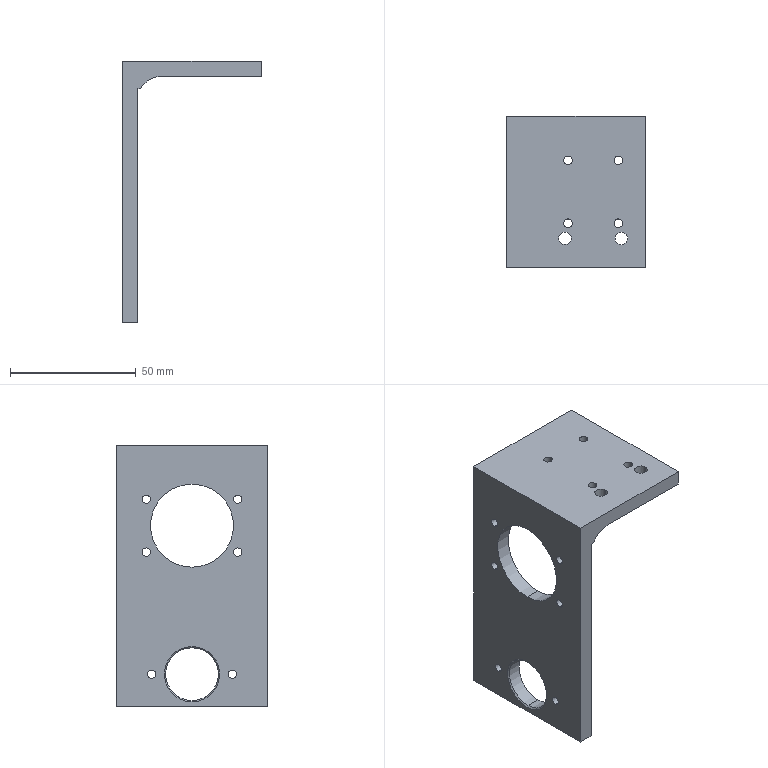Part | SolidWorks | features ICE 3, HoleWzd 2, Chamfer 1, Extrusion 1, Fillet 1 | 1 solid | 40 faces | box 55 x 60 x 104 mm | volume 48156 mm3 | cylinder 29 | plane 9 | cone 2 | commonest cylinder face diameters 3.3 x12 3.4 x8 5 x4 21 x2 33 x2 20 x1
STEP:
#1=CARTESIAN_POINT('',(0.5,30.,-101.5));
#2=VERTEX_POINT('',#1);
#3=CARTESIAN_POINT('',(0.5,30.,-80.5));
#4=VERTEX_POINT('',#3);
#5=CARTESIAN_POINT('',(0.5,30.,-91.));
#6=DIRECTION('',(-1.,0.,0.));
#7=DIRECTION('',(0.,0.,-1.));
#8=AXIS2_PLACEMENT_3D('',#5,#6,#7);
#9=CIRCLE('',#8,10.5);
#10=EDGE_CURVE('',#2,#4,#9,.T.);
#11=ORIENTED_EDGE('',*,*,#10,.F.);
#12=CARTESIAN_POINT('',(0.,30.,-102.));
#13=VERTEX_POINT('',#12);
#14=CARTESIAN_POINT('',(0.5,30.,-101.5));
#15=DIRECTION('',(-0.7071,0.,-0.7071));
#16=VECTOR('',#15,1000.);
#17=LINE('',#14,#16);
#18=EDGE_CURVE('',#2,#13,#17,.T.);
#19=ORIENTED_EDGE('',*,*,#18,.T.);
#20=CARTESIAN_POINT('',(0.,30.,-80.));
#21=VERTEX_POINT('',#20);
#22=CARTESIAN_POINT('',(0.,30.,-91.));
#23=DIRECTION('',(1.,0.,0.));
#24=DIRECTION('',(0.,0.,-1.));
#25=AXIS2_PLACEMENT_3D('',#22,#23,#24);
#26=CIRCLE('',#25,11.);
#27=EDGE_CURVE('',#21,#13,#26,.T.);
#28=ORIENTED_EDGE('',*,*,#27,.F.);
#29=CARTESIAN_POINT('',(0.5,30.,-80.5));
#30=DIRECTION('',(-0.7071,0.,0.7071));
#31=VECTOR('',#30,1000.);
#32=LINE('',#29,#31);
#33=EDGE_CURVE('',#4,#21,#32,.T.);
#34=ORIENTED_EDGE('',*,*,#33,.F.);
#35=EDGE_LOOP('',(#11,#19,#28,#34));
#36=FACE_OUTER_BOUND('',#35,.T.);
#37=CARTESIAN_POINT('',(0.5,30.,-91.));
#38=DIRECTION('',(-1.,0.,0.));
#39=DIRECTION('',(0.,0.,1.));
#40=AXIS2_PLACEMENT_3D('',#37,#38,#39);
#41=CONICAL_SURFACE('',#40,10.5,0.7854);
#42=ADVANCED_FACE('',(#36),#41,.F.);
#43=CARTESIAN_POINT('',(6.,11.813,-19.85));
#44=VERTEX_POINT('',#43);
#45=CARTESIAN_POINT('',(6.,11.813,-23.15));
#46=VERTEX_POINT('',#45);
#47=CARTESIAN_POINT('',(6.,11.813,-21.5));
#48=DIRECTION('',(1.,0.,0.));
#49=DIRECTION('',(0.,0.,-1.));
#50=AXIS2_PLACEMENT_3D('',#47,#48,#49);
#51=CIRCLE('',#50,1.65);
#52=EDGE_CURVE('',#44,#46,#51,.T.);
#53=ORIENTED_EDGE('',*,*,#52,.T.);
#54=CARTESIAN_POINT('',(0.,11.813,-23.15));
#55=VERTEX_POINT('',#54);
#56=CARTESIAN_POINT('',(0.,11.813,-23.15));
#57=DIRECTION('',(-1.,0.,0.));
#58=VECTOR('',#57,1000.);
#59=LINE('',#56,#58);
#60=EDGE_CURVE('',#46,#55,#59,.T.);
#61=ORIENTED_EDGE('',*,*,#60,.T.);
#62=CARTESIAN_POINT('',(0.,11.813,-19.85));
#63=VERTEX_POINT('',#62);
#64=CARTESIAN_POINT('',(0.,11.813,-21.5));
#65=DIRECTION('',(-1.,0.,0.));
#66=DIRECTION('',(0.,0.,1.));
#67=AXIS2_PLACEMENT_3D('',#64,#65,#66);
#68=CIRCLE('',#67,1.65);
#69=EDGE_CURVE('',#55,#63,#68,.T.);
#70=ORIENTED_EDGE('',*,*,#69,.T.);
#71=CARTESIAN_POINT('',(0.,11.813,-19.85));
#72=DIRECTION('',(-1.,0.,0.));
#73=VECTOR('',#72,1000.);
#74=LINE('',#71,#73);
#75=EDGE_CURVE('',#44,#63,#74,.T.);
#76=ORIENTED_EDGE('',*,*,#75,.F.);
#77=EDGE_LOOP('',(#53,#61,#70,#76));
#78=FACE_OUTER_BOUND('',#77,.T.);
#79=CARTESIAN_POINT('',(0.,11.813,-21.5));
#80=DIRECTION('',(-1.,0.,0.));
#81=DIRECTION('',(0.,0.,1.));
#82=AXIS2_PLACEMENT_3D('',#79,#80,#81);
#83=CYLINDRICAL_SURFACE('',#82,1.65);
#84=ADVANCED_FACE('',(#78),#83,.F.);
#85=CARTESIAN_POINT('',(6.,46.,-89.35));
#86=VERTEX_POINT('',#85);
#87=CARTESIAN_POINT('',(6.,46.,-92.65));
#88=VERTEX_POINT('',#87);
#89=CARTESIAN_POINT('',(6.,46.,-91.));
#90=DIRECTION('',(1.,0.,0.));
#91=DIRECTION('',(0.,0.,-1.));
#92=AXIS2_PLACEMENT_3D('',#89,#90,#91);
#93=CIRCLE('',#92,1.65);
#94=EDGE_CURVE('',#86,#88,#93,.T.);
#95=ORIENTED_EDGE('',*,*,#94,.T.);
#96=CARTESIAN_POINT('',(0.,46.,-92.65));
#97=VERTEX_POINT('',#96);
#98=CARTESIAN_POINT('',(0.,46.,-92.65));
#99=DIRECTION('',(-1.,0.,0.));
#100=VECTOR('',#99,1000.);
#101=LINE('',#98,#100);
#102=EDGE_CURVE('',#88,#97,#101,.T.);
#103=ORIENTED_EDGE('',*,*,#102,.T.);
#104=CARTESIAN_POINT('',(0.,46.,-89.35));
#105=VERTEX_POINT('',#104);
#106=CARTESIAN_POINT('',(0.,46.,-91.));
#107=DIRECTION('',(-1.,0.,0.));
#108=DIRECTION('',(0.,0.,1.));
#109=AXIS2_PLACEMENT_3D('',#106,#107,#108);
#110=CIRCLE('',#109,1.65);
#111=EDGE_CURVE('',#97,#105,#110,.T.);
#112=ORIENTED_EDGE('',*,*,#111,.T.);
#113=CARTESIAN_POINT('',(0.,46.,-89.35));
#114=DIRECTION('',(-1.,0.,0.));
#115=VECTOR('',#114,1000.);
#116=LINE('',#113,#115);
#117=EDGE_CURVE('',#86,#105,#116,.T.);
#118=ORIENTED_EDGE('',*,*,#117,.F.);
#119=EDGE_LOOP('',(#95,#103,#112,#118));
#120=FACE_OUTER_BOUND('',#119,.T.);
#121=CARTESIAN_POINT('',(0.,46.,-91.));
#122=DIRECTION('',(-1.,0.,0.));
#123=DIRECTION('',(0.,0.,1.));
#124=AXIS2_PLACEMENT_3D('',#121,#122,#123);
#125=CYLINDRICAL_SURFACE('',#124,1.65);
#126=ADVANCED_FACE('',(#120),#125,.F.);
#127=CARTESIAN_POINT('',(6.,14.,-89.35));
#128=VERTEX_POINT('',#127);
#129=CARTESIAN_POINT('',(6.,14.,-92.65));
#130=VERTEX_POINT('',#129);
#131=CARTESIAN_POINT('',(6.,14.,-91.));
#132=DIRECTION('',(1.,0.,0.));
#133=DIRECTION('',(0.,0.,-1.));
#134=AXIS2_PLACEMENT_3D('',#131,#132,#133);
#135=CIRCLE('',#134,1.65);
#136=EDGE_CURVE('',#128,#130,#135,.T.);
#137=ORIENTED_EDGE('',*,*,#136,.T.);
#138=CARTESIAN_POINT('',(0.,14.,-92.65));
#139=VERTEX_POINT('',#138);
#140=CARTESIAN_POINT('',(0.,14.,-92.65));
#141=DIRECTION('',(-1.,0.,0.));
#142=VECTOR('',#141,1000.);
#143=LINE('',#140,#142);
#144=EDGE_CURVE('',#130,#139,#143,.T.);
#145=ORIENTED_EDGE('',*,*,#144,.T.);
#146=CARTESIAN_POINT('',(0.,14.,-89.35));
#147=VERTEX_POINT('',#146);
#148=CARTESIAN_POINT('',(0.,14.,-91.));
#149=DIRECTION('',(-1.,0.,0.));
#150=DIRECTION('',(0.,0.,1.));
#151=AXIS2_PLACEMENT_3D('',#148,#149,#150);
#152=CIRCLE('',#151,1.65);
#153=EDGE_CURVE('',#139,#147,#152,.T.);
#154=ORIENTED_EDGE('',*,*,#153,.T.);
#155=CARTESIAN_POINT('',(0.,14.,-89.35));
#156=DIRECTION('',(-1.,0.,0.));
#157=VECTOR('',#156,1000.);
#158=LINE('',#155,#157);
#159=EDGE_CURVE('',#128,#147,#158,.T.);
#160=ORIENTED_EDGE('',*,*,#159,.F.);
#161=EDGE_LOOP('',(#137,#145,#154,#160));
#162=FACE_OUTER_BOUND('',#161,.T.);
#163=CARTESIAN_POINT('',(0.,14.,-91.));
#164=DIRECTION('',(-1.,0.,0.));
#165=DIRECTION('',(0.,0.,1.));
#166=AXIS2_PLACEMENT_3D('',#163,#164,#165);
#167=CYLINDRICAL_SURFACE('',#166,1.65);
#168=ADVANCED_FACE('',(#162),#167,.F.);
#169=CARTESIAN_POINT('',(6.,48.187,-19.85));
#170=VERTEX_POINT('',#169);
#171=CARTESIAN_POINT('',(6.,48.187,-23.15));
#172=VERTEX_POINT('',#171);
#173=CARTESIAN_POINT('',(6.,48.187,-21.5));
#174=DIRECTION('',(1.,0.,0.));
#175=DIRECTION('',(0.,0.,-1.));
#176=AXIS2_PLACEMENT_3D('',#173,#174,#175);
#177=CIRCLE('',#176,1.65);
#178=EDGE_CURVE('',#170,#172,#177,.T.);
#179=ORIENTED_EDGE('',*,*,#178,.T.);
#180=CARTESIAN_POINT('',(0.,48.187,-23.15));
#181=VERTEX_POINT('',#180);
#182=CARTESIAN_POINT('',(0.,48.187,-23.15));
#183=DIRECTION('',(-1.,0.,0.));
#184=VECTOR('',#183,1000.);
#185=LINE('',#182,#184);
#186=EDGE_CURVE('',#172,#181,#185,.T.);
#187=ORIENTED_EDGE('',*,*,#186,.T.);
#188=CARTESIAN_POINT('',(0.,48.187,-19.85));
#189=VERTEX_POINT('',#188);
#190=CARTESIAN_POINT('',(0.,48.187,-21.5));
#191=DIRECTION('',(-1.,0.,0.));
#192=DIRECTION('',(0.,0.,1.));
#193=AXIS2_PLACEMENT_3D('',#190,#191,#192);
#194=CIRCLE('',#193,1.65);
#195=EDGE_CURVE('',#181,#189,#194,.T.);
#196=ORIENTED_EDGE('',*,*,#195,.T.);
#197=CARTESIAN_POINT('',(0.,48.187,-19.85));
#198=DIRECTION('',(-1.,0.,0.));
#199=VECTOR('',#198,1000.);
#200=LINE('',#197,#199);
#201=EDGE_CURVE('',#170,#189,#200,.T.);
#202=ORIENTED_EDGE('',*,*,#201,.F.);
#203=EDGE_LOOP('',(#179,#187,#196,#202));
#204=FACE_OUTER_BOUND('',#203,.T.);
#205=CARTESIAN_POINT('',(0.,48.187,-21.5));
#206=DIRECTION('',(-1.,0.,0.));
#207=DIRECTION('',(0.,0.,1.));
#208=AXIS2_PLACEMENT_3D('',#205,#206,#207);
#209=CYLINDRICAL_SURFACE('',#208,1.65);
#210=ADVANCED_FACE('',(#204),#209,.F.);
#211=CARTESIAN_POINT('',(6.,48.187,-40.85));
#212=VERTEX_POINT('',#211);
#213=CARTESIAN_POINT('',(6.,48.187,-44.15));
#214=VERTEX_POINT('',#213);
#215=CARTESIAN_POINT('',(6.,48.187,-42.5));
#216=DIRECTION('',(1.,0.,0.));
#217=DIRECTION('',(0.,0.,-1.));
#218=AXIS2_PLACEMENT_3D('',#215,#216,#217);
#219=CIRCLE('',#218,1.65);
#220=EDGE_CURVE('',#212,#214,#219,.T.);
#221=ORIENTED_EDGE('',*,*,#220,.T.);
#222=CARTESIAN_POINT('',(0.,48.187,-44.15));
#223=VERTEX_POINT('',#222);
#224=CARTESIAN_POINT('',(0.,48.187,-44.15));
#225=DIRECTION('',(-1.,0.,0.));
#226=VECTOR('',#225,1000.);
#227=LINE('',#224,#226);
#228=EDGE_CURVE('',#214,#223,#227,.T.);
#229=ORIENTED_EDGE('',*,*,#228,.T.);
#230=CARTESIAN_POINT('',(0.,48.187,-40.85));
#231=VERTEX_POINT('',#230);
#232=CARTESIAN_POINT('',(0.,48.187,-42.5));
#233=DIRECTION('',(-1.,0.,0.));
#234=DIRECTION('',(0.,0.,1.));
#235=AXIS2_PLACEMENT_3D('',#232,#233,#234);
#236=CIRCLE('',#235,1.65);
#237=EDGE_CURVE('',#223,#231,#236,.T.);
#238=ORIENTED_EDGE('',*,*,#237,.T.);
#239=CARTESIAN_POINT('',(0.,48.187,-40.85));
#240=DIRECTION('',(-1.,0.,0.));
#241=VECTOR('',#240,1000.);
#242=LINE('',#239,#241);
#243=EDGE_CURVE('',#212,#231,#242,.T.);
#244=ORIENTED_EDGE('',*,*,#243,.F.);
#245=EDGE_LOOP('',(#221,#229,#238,#244));
#246=FACE_OUTER_BOUND('',#245,.T.);
#247=CARTESIAN_POINT('',(0.,48.187,-42.5));
#248=DIRECTION('',(-1.,0.,0.));
#249=DIRECTION('',(0.,0.,1.));
#250=AXIS2_PLACEMENT_3D('',#247,#248,#249);
#251=CYLINDRICAL_SURFACE('',#250,1.65);
#252=ADVANCED_FACE('',(#246),#251,.F.);
#253=CARTESIAN_POINT('',(6.,11.813,-40.85));
#254=VERTEX_POINT('',#253);
#255=CARTESIAN_POINT('',(6.,11.813,-44.15));
#256=VERTEX_POINT('',#255);
#257=CARTESIAN_POINT('',(6.,11.813,-42.5));
#258=DIRECTION('',(1.,0.,0.));
#259=DIRECTION('',(0.,0.,-1.));
#260=AXIS2_PLACEMENT_3D('',#257,#258,#259);
#261=CIRCLE('',#260,1.65);
#262=EDGE_CURVE('',#254,#256,#261,.T.);
#263=ORIENTED_EDGE('',*,*,#262,.T.);
#264=CARTESIAN_POINT('',(0.,11.813,-44.15));
#265=VERTEX_POINT('',#264);
#266=CARTESIAN_POINT('',(0.,11.813,-44.15));
#267=DIRECTION('',(-1.,0.,0.));
#268=VECTOR('',#267,1000.);
#269=LINE('',#266,#268);
#270=EDGE_CURVE('',#256,#265,#269,.T.);
#271=ORIENTED_EDGE('',*,*,#270,.T.);
#272=CARTESIAN_POINT('',(0.,11.813,-40.85));
#273=VERTEX_POINT('',#272);
#274=CARTESIAN_POINT('',(0.,11.813,-42.5));
#275=DIRECTION('',(-1.,0.,0.));
#276=DIRECTION('',(0.,0.,1.));
#277=AXIS2_PLACEMENT_3D('',#274,#275,#276);
#278=CIRCLE('',#277,1.65);
#279=EDGE_CURVE('',#265,#273,#278,.T.);
#280=ORIENTED_EDGE('',*,*,#279,.T.);
#281=CARTESIAN_POINT('',(0.,11.813,-40.85));
#282=DIRECTION('',(-1.,0.,0.));
#283=VECTOR('',#282,1000.);
#284=LINE('',#281,#283);
#285=EDGE_CURVE('',#254,#273,#284,.T.);
#286=ORIENTED_EDGE('',*,*,#285,.F.);
#287=EDGE_LOOP('',(#263,#271,#280,#286));
#288=FACE_OUTER_BOUND('',#287,.T.);
#289=CARTESIAN_POINT('',(0.,11.813,-42.5));
#290=DIRECTION('',(-1.,0.,0.));
#291=DIRECTION('',(0.,0.,1.));
#292=AXIS2_PLACEMENT_3D('',#289,#290,#291);
#293=CYLINDRICAL_SURFACE('',#292,1.65);
#294=ADVANCED_FACE('',(#288),#293,.F.);
#295=CARTESIAN_POINT('',(6.,30.,-80.5));
#296=VERTEX_POINT('',#295);
#297=CARTESIAN_POINT('',(6.,30.,-101.5));
#298=VERTEX_POINT('',#297);
#299=CARTESIAN_POINT('',(6.,30.,-91.));
#300=DIRECTION('',(1.,0.,0.));
#301=DIRECTION('',(0.,0.,-1.));
#302=AXIS2_PLACEMENT_3D('',#299,#300,#301);
#303=CIRCLE('',#302,10.5);
#304=EDGE_CURVE('',#296,#298,#303,.T.);
#305=ORIENTED_EDGE('',*,*,#304,.T.);
#306=CARTESIAN_POINT('',(55.,30.,-101.5));
#307=DIRECTION('',(-1.,0.,0.));
#308=VECTOR('',#307,1000.);
#309=LINE('',#306,#308);
#310=EDGE_CURVE('',#298,#2,#309,.T.);
#311=ORIENTED_EDGE('',*,*,#310,.T.);
#312=ORIENTED_EDGE('',*,*,#10,.T.);
#313=CARTESIAN_POINT('',(55.,30.,-80.5));
#314=DIRECTION('',(-1.,0.,0.));
#315=VECTOR('',#314,1000.);
#316=LINE('',#313,#315);
#317=EDGE_CURVE('',#296,#4,#316,.T.);
#318=ORIENTED_EDGE('',*,*,#317,.F.);
#319=EDGE_LOOP('',(#305,#311,#312,#318));
#320=FACE_OUTER_BOUND('',#319,.T.);
#321=CARTESIAN_POINT('',(55.,30.,-91.));
#322=DIRECTION('',(-1.,0.,0.));
#323=DIRECTION('',(0.,0.,1.));
#324=AXIS2_PLACEMENT_3D('',#321,#322,#323);
#325=CYLINDRICAL_SURFACE('',#324,10.5);
#326=ADVANCED_FACE('',(#320),#325,.F.);
#327=CARTESIAN_POINT('',(6.,30.,-15.5));
#328=VERTEX_POINT('',#327);
#329=CARTESIAN_POINT('',(6.,30.,-48.5));
#330=VERTEX_POINT('',#329);
#331=CARTESIAN_POINT('',(6.,30.,-32.));
#332=DIRECTION('',(1.,0.,0.));
#333=DIRECTION('',(0.,0.,-1.));
#334=AXIS2_PLACEMENT_3D('',#331,#332,#333);
#335=CIRCLE('',#334,16.5);
#336=EDGE_CURVE('',#328,#330,#335,.T.);
#337=ORIENTED_EDGE('',*,*,#336,.T.);
#338=CARTESIAN_POINT('',(0.,30.,-48.5));
#339=VERTEX_POINT('',#338);
#340=CARTESIAN_POINT('',(55.,30.,-48.5));
#341=DIRECTION('',(-1.,0.,0.));
#342=VECTOR('',#341,1000.);
#343=LINE('',#340,#342);
#344=EDGE_CURVE('',#330,#339,#343,.T.);
#345=ORIENTED_EDGE('',*,*,#344,.T.);
#346=CARTESIAN_POINT('',(0.,30.,-15.5));
#347=VERTEX_POINT('',#346);
#348=CARTESIAN_POINT('',(0.,30.,-32.));
#349=DIRECTION('',(-1.,0.,0.));
#350=DIRECTION('',(0.,0.,1.));
#351=AXIS2_PLACEMENT_3D('',#348,#349,#350);
#352=CIRCLE('',#351,16.5);
#353=EDGE_CURVE('',#339,#347,#352,.T.);
#354=ORIENTED_EDGE('',*,*,#353,.T.);
#355=CARTESIAN_POINT('',(55.,30.,-15.5));
#356=DIRECTION('',(-1.,0.,0.));
#357=VECTOR('',#356,1000.);
#358=LINE('',#355,#357);
#359=EDGE_CURVE('',#328,#347,#358,.T.);
#360=ORIENTED_EDGE('',*,*,#359,.F.);
#361=EDGE_LOOP('',(#337,#345,#354,#360));
#362=FACE_OUTER_BOUND('',#361,.T.);
#363=CARTESIAN_POINT('',(55.,30.,-32.));
#364=DIRECTION('',(-1.,0.,0.));
#365=DIRECTION('',(0.,0.,1.));
#366=AXIS2_PLACEMENT_3D('',#363,#364,#365);
#367=CYLINDRICAL_SURFACE('',#366,16.5);
#368=ADVANCED_FACE('',(#362),#367,.F.);
#369=CARTESIAN_POINT('',(43.,11.5,-6.));
#370=VERTEX_POINT('',#369);
#371=CARTESIAN_POINT('',(48.,11.5,-6.));
#372=VERTEX_POINT('',#371);
#373=CARTESIAN_POINT('',(45.5,11.5,-6.));
#374=DIRECTION('',(0.,0.,1.));
#375=DIRECTION('',(1.,0.,0.));
#376=AXIS2_PLACEMENT_3D('',#373,#374,#375);
#377=CIRCLE('',#376,2.5);
#378=EDGE_CURVE('',#370,#372,#377,.T.);
#379=ORIENTED_EDGE('',*,*,#378,.F.);
#380=CARTESIAN_POINT('',(43.,11.5,0.));
#381=VERTEX_POINT('',#380);
#382=CARTESIAN_POINT('',(43.,11.5,-104.));
#383=DIRECTION('',(0.,0.,1.));
#384=VECTOR('',#383,1000.);
#385=LINE('',#382,#384);
#386=EDGE_CURVE('',#370,#381,#385,.T.);
#387=ORIENTED_EDGE('',*,*,#386,.T.);
#388=CARTESIAN_POINT('',(48.,11.5,0.));
#389=VERTEX_POINT('',#388);
#390=CARTESIAN_POINT('',(45.5,11.5,0.));
#391=DIRECTION('',(0.,0.,1.));
#392=DIRECTION('',(1.,0.,0.));
#393=AXIS2_PLACEMENT_3D('',#390,#391,#392);
#394=CIRCLE('',#393,2.5);
#395=EDGE_CURVE('',#381,#389,#394,.T.);
#396=ORIENTED_EDGE('',*,*,#395,.T.);
#397=CARTESIAN_POINT('',(48.,11.5,-104.));
#398=DIRECTION('',(0.,0.,1.));
#399=VECTOR('',#398,1000.);
#400=LINE('',#397,#399);
#401=EDGE_CURVE('',#372,#389,#400,.T.);
#402=ORIENTED_EDGE('',*,*,#401,.F.);
#403=EDGE_LOOP('',(#379,#387,#396,#402));
#404=FACE_OUTER_BOUND('',#403,.T.);
#405=CARTESIAN_POINT('',(45.5,11.5,-104.));
#406=DIRECTION('',(0.,0.,1.));
#407=DIRECTION('',(1.,0.,0.));
#408=AXIS2_PLACEMENT_3D('',#405,#406,#407);
#409=CYLINDRICAL_SURFACE('',#408,2.5);
#410=ADVANCED_FACE('',(#404),#409,.F.);
#411=CARTESIAN_POINT('',(20.6,11.5,-6.));
#412=VERTEX_POINT('',#411);
#413=CARTESIAN_POINT('',(25.6,11.5,-6.));
#414=VERTEX_POINT('',#413);
#415=CARTESIAN_POINT('',(23.1,11.5,-6.));
#416=DIRECTION('',(0.,0.,1.));
#417=DIRECTION('',(1.,0.,0.));
#418=AXIS2_PLACEMENT_3D('',#415,#416,#417);
#419=CIRCLE('',#418,2.5);
#420=EDGE_CURVE('',#412,#414,#419,.T.);
#421=ORIENTED_EDGE('',*,*,#420,.F.);
#422=CARTESIAN_POINT('',(20.6,11.5,0.));
#423=VERTEX_POINT('',#422);
#424=CARTESIAN_POINT('',(20.6,11.5,-104.));
#425=DIRECTION('',(0.,0.,1.));
#426=VECTOR('',#425,1000.);
#427=LINE('',#424,#426);
#428=EDGE_CURVE('',#412,#423,#427,.T.);
#429=ORIENTED_EDGE('',*,*,#428,.T.);
#430=CARTESIAN_POINT('',(25.6,11.5,0.));
#431=VERTEX_POINT('',#430);
#432=CARTESIAN_POINT('',(23.1,11.5,0.));
#433=DIRECTION('',(0.,0.,1.));
#434=DIRECTION('',(1.,0.,0.));
#435=AXIS2_PLACEMENT_3D('',#432,#433,#434);
#436=CIRCLE('',#435,2.5);
#437=EDGE_CURVE('',#423,#431,#436,.T.);
#438=ORIENTED_EDGE('',*,*,#437,.T.);
#439=CARTESIAN_POINT('',(25.6,11.5,-104.));
#440=DIRECTION('',(0.,0.,1.));
#441=VECTOR('',#440,1000.);
#442=LINE('',#439,#441);
#443=EDGE_CURVE('',#414,#431,#442,.T.);
#444=ORIENTED_EDGE('',*,*,#443,.F.);
#445=EDGE_LOOP('',(#421,#429,#438,#444));
#446=FACE_OUTER_BOUND('',#445,.T.);
#447=CARTESIAN_POINT('',(23.1,11.5,-104.));
#448=DIRECTION('',(0.,0.,1.));
#449=DIRECTION('',(1.,0.,0.));
#450=AXIS2_PLACEMENT_3D('',#447,#448,#449);
#451=CYLINDRICAL_SURFACE('',#450,2.5);
#452=ADVANCED_FACE('',(#446),#451,.F.);
#453=CARTESIAN_POINT('',(22.6,42.5,-6.));
#454=VERTEX_POINT('',#453);
#455=CARTESIAN_POINT('',(26.,42.5,-6.));
#456=VERTEX_POINT('',#455);
#457=CARTESIAN_POINT('',(24.3,42.5,-6.));
#458=DIRECTION('',(0.,0.,1.));
#459=DIRECTION('',(1.,0.,0.));
#460=AXIS2_PLACEMENT_3D('',#457,#458,#459);
#461=CIRCLE('',#460,1.7);
#462=EDGE_CURVE('',#454,#456,#461,.T.);
#463=ORIENTED_EDGE('',*,*,#462,.F.);
#464=CARTESIAN_POINT('',(22.6,42.5,0.));
#465=VERTEX_POINT('',#464);
#466=CARTESIAN_POINT('',(22.6,42.5,0.));
#467=DIRECTION('',(0.,0.,1.));
#468=VECTOR('',#467,1000.);
#469=LINE('',#466,#468);
#470=EDGE_CURVE('',#454,#465,#469,.T.);
#471=ORIENTED_EDGE('',*,*,#470,.T.);
#472=CARTESIAN_POINT('',(26.,42.5,0.));
#473=VERTEX_POINT('',#472);
#474=CARTESIAN_POINT('',(24.3,42.5,0.));
#475=DIRECTION('',(0.,0.,1.));
#476=DIRECTION('',(1.,0.,0.));
#477=AXIS2_PLACEMENT_3D('',#474,#475,#476);
#478=CIRCLE('',#477,1.7);
#479=EDGE_CURVE('',#465,#473,#478,.T.);
#480=ORIENTED_EDGE('',*,*,#479,.T.);
#481=CARTESIAN_POINT('',(26.,42.5,0.));
#482=DIRECTION('',(0.,0.,1.));
#483=VECTOR('',#482,1000.);
#484=LINE('',#481,#483);
#485=EDGE_CURVE('',#456,#473,#484,.T.);
#486=ORIENTED_EDGE('',*,*,#485,.F.);
#487=EDGE_LOOP('',(#463,#471,#480,#486));
#488=FACE_OUTER_BOUND('',#487,.T.);
#489=CARTESIAN_POINT('',(24.3,42.5,0.));
#490=DIRECTION('',(0.,0.,1.));
#491=DIRECTION('',(1.,0.,0.));
#492=AXIS2_PLACEMENT_3D('',#489,#490,#491);
#493=CYLINDRICAL_SURFACE('',#492,1.7);
#494=ADVANCED_FACE('',(#488),#493,.F.);
#495=CARTESIAN_POINT('',(42.6,42.5,-6.));
#496=VERTEX_POINT('',#495);
#497=CARTESIAN_POINT('',(46.,42.5,-6.));
#498=VERTEX_POINT('',#497);
#499=CARTESIAN_POINT('',(44.3,42.5,-6.));
#500=DIRECTION('',(0.,0.,1.));
#501=DIRECTION('',(1.,0.,0.));
#502=AXIS2_PLACEMENT_3D('',#499,#500,#501);
#503=CIRCLE('',#502,1.7);
#504=EDGE_CURVE('',#496,#498,#503,.T.);
#505=ORIENTED_EDGE('',*,*,#504,.F.);
#506=CARTESIAN_POINT('',(42.6,42.5,0.));
#507=VERTEX_POINT('',#506);
#508=CARTESIAN_POINT('',(42.6,42.5,0.));
#509=DIRECTION('',(0.,0.,1.));
#510=VECTOR('',#509,1000.);
#511=LINE('',#508,#510);
#512=EDGE_CURVE('',#496,#507,#511,.T.);
#513=ORIENTED_EDGE('',*,*,#512,.T.);
#514=CARTESIAN_POINT('',(46.,42.5,0.));
#515=VERTEX_POINT('',#514);
#516=CARTESIAN_POINT('',(44.3,42.5,0.));
#517=DIRECTION('',(0.,0.,1.));
#518=DIRECTION('',(1.,0.,0.));
#519=AXIS2_PLACEMENT_3D('',#516,#517,#518);
#520=CIRCLE('',#519,1.7);
#521=EDGE_CURVE('',#507,#515,#520,.T.);
#522=ORIENTED_EDGE('',*,*,#521,.T.);
#523=CARTESIAN_POINT('',(46.,42.5,0.));
#524=DIRECTION('',(0.,0.,1.));
#525=VECTOR('',#524,1000.);
#526=LINE('',#523,#525);
#527=EDGE_CURVE('',#498,#515,#526,.T.);
#528=ORIENTED_EDGE('',*,*,#527,.F.);
#529=EDGE_LOOP('',(#505,#513,#522,#528));
#530=FACE_OUTER_BOUND('',#529,.T.);
#531=CARTESIAN_POINT('',(44.3,42.5,0.));
#532=DIRECTION('',(0.,0.,1.));
#533=DIRECTION('',(1.,0.,0.));
#534=AXIS2_PLACEMENT_3D('',#531,#532,#533);
#535=CYLINDRICAL_SURFACE('',#534,1.7);
#536=ADVANCED_FACE('',(#530),#535,.F.);
#537=CARTESIAN_POINT('',(42.6,17.5,-6.));
#538=VERTEX_POINT('',#537);
#539=CARTESIAN_POINT('',(46.,17.5,-6.));
#540=VERTEX_POINT('',#539);
#541=CARTESIAN_POINT('',(44.3,17.5,-6.));
#542=DIRECTION('',(0.,0.,1.));
#543=DIRECTION('',(1.,0.,0.));
#544=AXIS2_PLACEMENT_3D('',#541,#542,#543);
#545=CIRCLE('',#544,1.7);
#546=EDGE_CURVE('',#538,#540,#545,.T.);
#547=ORIENTED_EDGE('',*,*,#546,.F.);
#548=CARTESIAN_POINT('',(42.6,17.5,0.));
#549=VERTEX_POINT('',#548);
#550=CARTESIAN_POINT('',(42.6,17.5,0.));
#551=DIRECTION('',(0.,0.,1.));
#552=VECTOR('',#551,1000.);
#553=LINE('',#550,#552);
#554=EDGE_CURVE('',#538,#549,#553,.T.);
#555=ORIENTED_EDGE('',*,*,#554,.T.);
#556=CARTESIAN_POINT('',(46.,17.5,0.));
#557=VERTEX_POINT('',#556);
#558=CARTESIAN_POINT('',(44.3,17.5,0.));
#559=DIRECTION('',(0.,0.,1.));
#560=DIRECTION('',(1.,0.,0.));
#561=AXIS2_PLACEMENT_3D('',#558,#559,#560);
#562=CIRCLE('',#561,1.7);
#563=EDGE_CURVE('',#549,#557,#562,.T.);
#564=ORIENTED_EDGE('',*,*,#563,.T.);
#565=CARTESIAN_POINT('',(46.,17.5,0.));
#566=DIRECTION('',(0.,0.,1.));
#567=VECTOR('',#566,1000.);
#568=LINE('',#565,#567);
#569=EDGE_CURVE('',#540,#557,#568,.T.);
#570=ORIENTED_EDGE('',*,*,#569,.F.);
#571=EDGE_LOOP('',(#547,#555,#564,#570));
#572=FACE_OUTER_BOUND('',#571,.T.);
#573=CARTESIAN_POINT('',(44.3,17.5,0.));
#574=DIRECTION('',(0.,0.,1.));
#575=DIRECTION('',(1.,0.,0.));
#576=AXIS2_PLACEMENT_3D('',#573,#574,#575);
#577=CYLINDRICAL_SURFACE('',#576,1.7);
#578=ADVANCED_FACE('',(#572),#577,.F.);
#579=CARTESIAN_POINT('',(22.6,17.5,-6.));
#580=VERTEX_POINT('',#579);
#581=CARTESIAN_POINT('',(26.,17.5,-6.));
#582=VERTEX_POINT('',#581);
#583=CARTESIAN_POINT('',(24.3,17.5,-6.));
#584=DIRECTION('',(0.,0.,1.));
#585=DIRECTION('',(1.,0.,0.));
#586=AXIS2_PLACEMENT_3D('',#583,#584,#585);
#587=CIRCLE('',#586,1.7);
#588=EDGE_CURVE('',#580,#582,#587,.T.);
#589=ORIENTED_EDGE('',*,*,#588,.F.);
#590=CARTESIAN_POINT('',(22.6,17.5,0.));
#591=VERTEX_POINT('',#590);
#592=CARTESIAN_POINT('',(22.6,17.5,0.));
#593=DIRECTION('',(0.,0.,1.));
#594=VECTOR('',#593,1000.);
#595=LINE('',#592,#594);
#596=EDGE_CURVE('',#580,#591,#595,.T.);
#597=ORIENTED_EDGE('',*,*,#596,.T.);
#598=CARTESIAN_POINT('',(26.,17.5,0.));
#599=VERTEX_POINT('',#598);
#600=CARTESIAN_POINT('',(24.3,17.5,0.));
#601=DIRECTION('',(0.,0.,1.));
#602=DIRECTION('',(1.,0.,0.));
#603=AXIS2_PLACEMENT_3D('',#600,#601,#602);
#604=CIRCLE('',#603,1.7);
#605=EDGE_CURVE('',#591,#599,#604,.T.);
#606=ORIENTED_EDGE('',*,*,#605,.T.);
#607=CARTESIAN_POINT('',(26.,17.5,0.));
#608=DIRECTION('',(0.,0.,1.));
#609=VECTOR('',#608,1000.);
#610=LINE('',#607,#609);
#611=EDGE_CURVE('',#582,#599,#610,.T.);
#612=ORIENTED_EDGE('',*,*,#611,.F.);
#613=EDGE_LOOP('',(#589,#597,#606,#612));
#614=FACE_OUTER_BOUND('',#613,.T.);
#615=CARTESIAN_POINT('',(24.3,17.5,0.));
#616=DIRECTION('',(0.,0.,1.));
#617=DIRECTION('',(1.,0.,0.));
#618=AXIS2_PLACEMENT_3D('',#615,#616,#617);
#619=CYLINDRICAL_SURFACE('',#618,1.7);
#620=ADVANCED_FACE('',(#614),#619,.F.);
#621=ORIENTED_EDGE('',*,*,#27,.T.);
#622=CARTESIAN_POINT('',(0.,30.,-91.));
#623=DIRECTION('',(1.,0.,0.));
#624=DIRECTION('',(0.,0.,-1.));
#625=AXIS2_PLACEMENT_3D('',#622,#623,#624);
#626=CIRCLE('',#625,11.);
#627=EDGE_CURVE('',#13,#21,#626,.T.);
#628=ORIENTED_EDGE('',*,*,#627,.T.);
#629=EDGE_LOOP('',(#621,#628));
#630=FACE_BOUND('',#629,.T.);
#631=CARTESIAN_POINT('',(0.,11.813,-21.5));
#632=DIRECTION('',(-1.,0.,0.));
#633=DIRECTION('',(0.,0.,1.));
#634=AXIS2_PLACEMENT_3D('',#631,#632,#633);
#635=CIRCLE('',#634,1.65);
#636=EDGE_CURVE('',#63,#55,#635,.T.);
#637=ORIENTED_EDGE('',*,*,#636,.F.);
#638=ORIENTED_EDGE('',*,*,#69,.F.);
#639=EDGE_LOOP('',(#637,#638));
#640=FACE_BOUND('',#639,.T.);
#641=CARTESIAN_POINT('',(0.,46.,-91.));
#642=DIRECTION('',(-1.,0.,0.));
#643=DIRECTION('',(0.,0.,1.));
#644=AXIS2_PLACEMENT_3D('',#641,#642,#643);
#645=CIRCLE('',#644,1.65);
#646=EDGE_CURVE('',#105,#97,#645,.T.);
#647=ORIENTED_EDGE('',*,*,#646,.F.);
#648=ORIENTED_EDGE('',*,*,#111,.F.);
#649=EDGE_LOOP('',(#647,#648));
#650=FACE_BOUND('',#649,.T.);
#651=CARTESIAN_POINT('',(0.,11.813,-42.5));
#652=DIRECTION('',(-1.,0.,0.));
#653=DIRECTION('',(0.,0.,1.));
#654=AXIS2_PLACEMENT_3D('',#651,#652,#653);
#655=CIRCLE('',#654,1.65);
#656=EDGE_CURVE('',#273,#265,#655,.T.);
#657=ORIENTED_EDGE('',*,*,#656,.F.);
#658=ORIENTED_EDGE('',*,*,#279,.F.);
#659=EDGE_LOOP('',(#657,#658));
#660=FACE_BOUND('',#659,.T.);
#661=CARTESIAN_POINT('',(0.,30.,-32.));
#662=DIRECTION('',(-1.,0.,0.));
#663=DIRECTION('',(0.,0.,1.));
#664=AXIS2_PLACEMENT_3D('',#661,#662,#663);
#665=CIRCLE('',#664,16.5);
#666=EDGE_CURVE('',#347,#339,#665,.T.);
#667=ORIENTED_EDGE('',*,*,#666,.F.);
#668=ORIENTED_EDGE('',*,*,#353,.F.);
#669=EDGE_LOOP('',(#667,#668));
#670=FACE_BOUND('',#669,.T.);
#671=CARTESIAN_POINT('',(0.,0.,-104.));
#672=VERTEX_POINT('',#671);
#673=CARTESIAN_POINT('',(0.,0.,0.));
#674=VERTEX_POINT('',#673);
#675=CARTESIAN_POINT('',(0.,0.,0.));
#676=DIRECTION('',(0.,0.,1.));
#677=VECTOR('',#676,1000.);
#678=LINE('',#675,#677);
#679=EDGE_CURVE('',#672,#674,#678,.T.);
#680=ORIENTED_EDGE('',*,*,#679,.T.);
#681=CARTESIAN_POINT('',(0.,60.,0.));
#682=VERTEX_POINT('',#681);
#683=CARTESIAN_POINT('',(0.,60.,0.));
#684=DIRECTION('',(0.,-1.,0.));
#685=VECTOR('',#684,1000.);
#686=LINE('',#683,#685);
#687=EDGE_CURVE('',#682,#674,#686,.T.);
#688=ORIENTED_EDGE('',*,*,#687,.F.);
#689=CARTESIAN_POINT('',(0.,60.,-104.));
#690=VERTEX_POINT('',#689);
#691=CARTESIAN_POINT('',(0.,60.,0.));
#692=DIRECTION('',(0.,0.,1.));
#693=VECTOR('',#692,1000.);
#694=LINE('',#691,#693);
#695=EDGE_CURVE('',#690,#682,#694,.T.);
#696=ORIENTED_EDGE('',*,*,#695,.F.);
#697=CARTESIAN_POINT('',(0.,60.,-104.));
#698=DIRECTION('',(0.,-1.,0.));
#699=VECTOR('',#698,1000.);
#700=LINE('',#697,#699);
#701=EDGE_CURVE('',#690,#672,#700,.T.);
#702=ORIENTED_EDGE('',*,*,#701,.T.);
#703=EDGE_LOOP('',(#680,#688,#696,#702));
#704=FACE_OUTER_BOUND('',#703,.T.);
#705=CARTESIAN_POINT('',(0.,48.187,-42.5));
#706=DIRECTION('',(-1.,0.,0.));
#707=DIRECTION('',(0.,0.,1.));
#708=AXIS2_PLACEMENT_3D('',#705,#706,#707);
#709=CIRCLE('',#708,1.65);
#710=EDGE_CURVE('',#231,#223,#709,.T.);
#711=ORIENTED_EDGE('',*,*,#710,.F.);
#712=ORIENTED_EDGE('',*,*,#237,.F.);
#713=EDGE_LOOP('',(#711,#712));
#714=FACE_BOUND('',#713,.T.);
#715=CARTESIAN_POINT('',(0.,48.187,-21.5));
#716=DIRECTION('',(-1.,0.,0.));
#717=DIRECTION('',(0.,0.,1.));
#718=AXIS2_PLACEMENT_3D('',#715,#716,#717);
#719=CIRCLE('',#718,1.65);
#720=EDGE_CURVE('',#189,#181,#719,.T.);
#721=ORIENTED_EDGE('',*,*,#720,.F.);
#722=ORIENTED_EDGE('',*,*,#195,.F.);
#723=EDGE_LOOP('',(#721,#722));
#724=FACE_BOUND('',#723,.T.);
#725=CARTESIAN_POINT('',(0.,14.,-91.));
#726=DIRECTION('',(-1.,0.,0.));
#727=DIRECTION('',(0.,0.,1.));
#728=AXIS2_PLACEMENT_3D('',#725,#726,#727);
#729=CIRCLE('',#728,1.65);
#730=EDGE_CURVE('',#147,#139,#729,.T.);
#731=ORIENTED_EDGE('',*,*,#730,.F.);
#732=ORIENTED_EDGE('',*,*,#153,.F.);
#733=EDGE_LOOP('',(#731,#732));
#734=FACE_BOUND('',#733,.T.);
#735=CARTESIAN_POINT('',(0.,60.,0.));
#736=DIRECTION('',(1.,0.,0.));
#737=DIRECTION('',(0.,0.,-1.));
#738=AXIS2_PLACEMENT_3D('',#735,#736,#737);
#739=PLANE('',#738);
#740=ADVANCED_FACE('',(#630,#640,#650,#660,#670,#704,#714,#724,#734),#739,.F.);
#741=CARTESIAN_POINT('',(45.5,11.5,0.));
#742=DIRECTION('',(0.,0.,1.));
#743=DIRECTION('',(1.,0.,0.));
#744=AXIS2_PLACEMENT_3D('',#741,#742,#743);
#745=CIRCLE('',#744,2.5);
#746=EDGE_CURVE('',#389,#381,#745,.T.);
#747=ORIENTED_EDGE('',*,*,#746,.F.);
#748=ORIENTED_EDGE('',*,*,#395,.F.);
#749=EDGE_LOOP('',(#747,#748));
#750=FACE_BOUND('',#749,.T.);
#751=CARTESIAN_POINT('',(23.1,11.5,0.));
#752=DIRECTION('',(0.,0.,1.));
#753=DIRECTION('',(1.,0.,0.));
#754=AXIS2_PLACEMENT_3D('',#751,#752,#753);
#755=CIRCLE('',#754,2.5);
#756=EDGE_CURVE('',#431,#423,#755,.T.);
#757=ORIENTED_EDGE('',*,*,#756,.F.);
#758=ORIENTED_EDGE('',*,*,#437,.F.);
#759=EDGE_LOOP('',(#757,#758));
#760=FACE_BOUND('',#759,.T.);
#761=CARTESIAN_POINT('',(24.3,42.5,0.));
#762=DIRECTION('',(0.,0.,1.));
#763=DIRECTION('',(1.,0.,0.));
#764=AXIS2_PLACEMENT_3D('',#761,#762,#763);
#765=CIRCLE('',#764,1.7);
#766=EDGE_CURVE('',#473,#465,#765,.T.);
#767=ORIENTED_EDGE('',*,*,#766,.F.);
#768=ORIENTED_EDGE('',*,*,#479,.F.);
#769=EDGE_LOOP('',(#767,#768));
#770=FACE_BOUND('',#769,.T.);
#771=CARTESIAN_POINT('',(24.3,17.5,0.));
#772=DIRECTION('',(0.,0.,1.));
#773=DIRECTION('',(1.,0.,0.));
#774=AXIS2_PLACEMENT_3D('',#771,#772,#773);
#775=CIRCLE('',#774,1.7);
#776=EDGE_CURVE('',#599,#591,#775,.T.);
#777=ORIENTED_EDGE('',*,*,#776,.F.);
#778=ORIENTED_EDGE('',*,*,#605,.F.);
#779=EDGE_LOOP('',(#777,#778));
#780=FACE_BOUND('',#779,.T.);
#781=CARTESIAN_POINT('',(55.,0.,0.));
#782=VERTEX_POINT('',#781);
#783=CARTESIAN_POINT('',(55.,0.,0.));
#784=DIRECTION('',(1.,0.,0.));
#785=VECTOR('',#784,1000.);
#786=LINE('',#783,#785);
#787=EDGE_CURVE('',#674,#782,#786,.T.);
#788=ORIENTED_EDGE('',*,*,#787,.T.);
#789=CARTESIAN_POINT('',(55.,60.,0.));
#790=VERTEX_POINT('',#789);
#791=CARTESIAN_POINT('',(55.,60.,0.));
#792=DIRECTION('',(0.,-1.,0.));
#793=VECTOR('',#792,1000.);
#794=LINE('',#791,#793);
#795=EDGE_CURVE('',#790,#782,#794,.T.);
#796=ORIENTED_EDGE('',*,*,#795,.F.);
#797=CARTESIAN_POINT('',(55.,60.,0.));
#798=DIRECTION('',(1.,0.,0.));
#799=VECTOR('',#798,1000.);
#800=LINE('',#797,#799);
#801=EDGE_CURVE('',#682,#790,#800,.T.);
#802=ORIENTED_EDGE('',*,*,#801,.F.);
#803=ORIENTED_EDGE('',*,*,#687,.T.);
#804=EDGE_LOOP('',(#788,#796,#802,#803));
#805=FACE_OUTER_BOUND('',#804,.T.);
#806=CARTESIAN_POINT('',(44.3,17.5,0.));
#807=DIRECTION('',(0.,0.,1.));
#808=DIRECTION('',(1.,0.,0.));
#809=AXIS2_PLACEMENT_3D('',#806,#807,#808);
#810=CIRCLE('',#809,1.7);
#811=EDGE_CURVE('',#557,#549,#810,.T.);
#812=ORIENTED_EDGE('',*,*,#811,.F.);
#813=ORIENTED_EDGE('',*,*,#563,.F.);
#814=EDGE_LOOP('',(#812,#813));
#815=FACE_BOUND('',#814,.T.);
#816=CARTESIAN_POINT('',(44.3,42.5,0.));
#817=DIRECTION('',(0.,0.,1.));
#818=DIRECTION('',(1.,0.,0.));
#819=AXIS2_PLACEMENT_3D('',#816,#817,#818);
#820=CIRCLE('',#819,1.7);
#821=EDGE_CURVE('',#515,#507,#820,.T.);
#822=ORIENTED_EDGE('',*,*,#821,.F.);
#823=ORIENTED_EDGE('',*,*,#521,.F.);
#824=EDGE_LOOP('',(#822,#823));
#825=FACE_BOUND('',#824,.T.);
#826=CARTESIAN_POINT('',(55.,60.,0.));
#827=DIRECTION('',(0.,0.,-1.));
#828=DIRECTION('',(-1.,0.,0.));
#829=AXIS2_PLACEMENT_3D('',#826,#827,#828);
#830=PLANE('',#829);
#831=ADVANCED_FACE('',(#750,#760,#770,#780,#805,#815,#825),#830,.F.);
#832=CARTESIAN_POINT('',(6.,0.,-104.));
#833=VERTEX_POINT('',#832);
#834=CARTESIAN_POINT('',(6.,60.,-104.));
#835=VERTEX_POINT('',#834);
#836=CARTESIAN_POINT('',(6.,60.,-104.));
#837=DIRECTION('',(0.,1.,0.));
#838=VECTOR('',#837,1000.);
#839=LINE('',#836,#838);
#840=EDGE_CURVE('',#833,#835,#839,.T.);
#841=ORIENTED_EDGE('',*,*,#840,.F.);
#842=CARTESIAN_POINT('',(0.,0.,-104.));
#843=DIRECTION('',(-1.,0.,0.));
#844=VECTOR('',#843,1000.);
#845=LINE('',#842,#844);
#846=EDGE_CURVE('',#833,#672,#845,.T.);
#847=ORIENTED_EDGE('',*,*,#846,.T.);
#848=ORIENTED_EDGE('',*,*,#701,.F.);
#849=CARTESIAN_POINT('',(0.,60.,-104.));
#850=DIRECTION('',(-1.,0.,0.));
#851=VECTOR('',#850,1000.);
#852=LINE('',#849,#851);
#853=EDGE_CURVE('',#835,#690,#852,.T.);
#854=ORIENTED_EDGE('',*,*,#853,.F.);
#855=EDGE_LOOP('',(#841,#847,#848,#854));
#856=FACE_OUTER_BOUND('',#855,.T.);
#857=CARTESIAN_POINT('',(0.,60.,-104.));
#858=DIRECTION('',(0.,0.,1.));
#859=DIRECTION('',(1.,0.,0.));
#860=AXIS2_PLACEMENT_3D('',#857,#858,#859);
#861=PLANE('',#860);
#862=ADVANCED_FACE('',(#856),#861,.F.);
#863=CARTESIAN_POINT('',(55.,0.,-6.));
#864=VERTEX_POINT('',#863);
#865=CARTESIAN_POINT('',(55.,0.,-6.));
#866=DIRECTION('',(0.,0.,-1.));
#867=VECTOR('',#866,1000.);
#868=LINE('',#865,#867);
#869=EDGE_CURVE('',#782,#864,#868,.T.);
#870=ORIENTED_EDGE('',*,*,#869,.T.);
#871=CARTESIAN_POINT('',(55.,60.,-6.));
#872=VERTEX_POINT('',#871);
#873=CARTESIAN_POINT('',(55.,60.,-6.));
#874=DIRECTION('',(0.,-1.,0.));
#875=VECTOR('',#874,1000.);
#876=LINE('',#873,#875);
#877=EDGE_CURVE('',#872,#864,#876,.T.);
#878=ORIENTED_EDGE('',*,*,#877,.F.);
#879=CARTESIAN_POINT('',(55.,60.,-6.));
#880=DIRECTION('',(0.,0.,-1.));
#881=VECTOR('',#880,1000.);
#882=LINE('',#879,#881);
#883=EDGE_CURVE('',#790,#872,#882,.T.);
#884=ORIENTED_EDGE('',*,*,#883,.F.);
#885=ORIENTED_EDGE('',*,*,#795,.T.);
#886=EDGE_LOOP('',(#870,#878,#884,#885));
#887=FACE_OUTER_BOUND('',#886,.T.);
#888=CARTESIAN_POINT('',(55.,60.,-6.));
#889=DIRECTION('',(-1.,0.,0.));
#890=DIRECTION('',(0.,0.,1.));
#891=AXIS2_PLACEMENT_3D('',#888,#889,#890);
#892=PLANE('',#891);
#893=ADVANCED_FACE('',(#887),#892,.F.);
#894=CARTESIAN_POINT('',(45.5,11.5,-6.));
#895=DIRECTION('',(0.,0.,1.));
#896=DIRECTION('',(1.,0.,0.));
#897=AXIS2_PLACEMENT_3D('',#894,#895,#896);
#898=CIRCLE('',#897,2.5);
#899=EDGE_CURVE('',#372,#370,#898,.T.);
#900=ORIENTED_EDGE('',*,*,#899,.T.);
#901=ORIENTED_EDGE('',*,*,#378,.T.);
#902=EDGE_LOOP('',(#900,#901));
#903=FACE_BOUND('',#902,.T.);
#904=CARTESIAN_POINT('',(23.1,11.5,-6.));
#905=DIRECTION('',(0.,0.,1.));
#906=DIRECTION('',(1.,0.,0.));
#907=AXIS2_PLACEMENT_3D('',#904,#905,#906);
#908=CIRCLE('',#907,2.5);
#909=EDGE_CURVE('',#414,#412,#908,.T.);
#910=ORIENTED_EDGE('',*,*,#909,.T.);
#911=ORIENTED_EDGE('',*,*,#420,.T.);
#912=EDGE_LOOP('',(#910,#911));
#913=FACE_BOUND('',#912,.T.);
#914=CARTESIAN_POINT('',(24.3,42.5,-6.));
#915=DIRECTION('',(0.,0.,1.));
#916=DIRECTION('',(1.,0.,0.));
#917=AXIS2_PLACEMENT_3D('',#914,#915,#916);
#918=CIRCLE('',#917,1.7);
#919=EDGE_CURVE('',#456,#454,#918,.T.);
#920=ORIENTED_EDGE('',*,*,#919,.T.);
#921=ORIENTED_EDGE('',*,*,#462,.T.);
#922=EDGE_LOOP('',(#920,#921));
#923=FACE_BOUND('',#922,.T.);
#924=CARTESIAN_POINT('',(44.3,42.5,-6.));
#925=DIRECTION('',(0.,0.,1.));
#926=DIRECTION('',(1.,0.,0.));
#927=AXIS2_PLACEMENT_3D('',#924,#925,#926);
#928=CIRCLE('',#927,1.7);
#929=EDGE_CURVE('',#498,#496,#928,.T.);
#930=ORIENTED_EDGE('',*,*,#929,.T.);
#931=ORIENTED_EDGE('',*,*,#504,.T.);
#932=EDGE_LOOP('',(#930,#931));
#933=FACE_BOUND('',#932,.T.);
#934=CARTESIAN_POINT('',(44.3,17.5,-6.));
#935=DIRECTION('',(0.,0.,1.));
#936=DIRECTION('',(1.,0.,0.));
#937=AXIS2_PLACEMENT_3D('',#934,#935,#936);
#938=CIRCLE('',#937,1.7);
#939=EDGE_CURVE('',#540,#538,#938,.T.);
#940=ORIENTED_EDGE('',*,*,#939,.T.);
#941=ORIENTED_EDGE('',*,*,#546,.T.);
#942=EDGE_LOOP('',(#940,#941));
#943=FACE_BOUND('',#942,.T.);
#944=CARTESIAN_POINT('',(24.3,17.5,-6.));
#945=DIRECTION('',(0.,0.,1.));
#946=DIRECTION('',(1.,0.,0.));
#947=AXIS2_PLACEMENT_3D('',#944,#945,#946);
#948=CIRCLE('',#947,1.7);
#949=EDGE_CURVE('',#582,#580,#948,.T.);
#950=ORIENTED_EDGE('',*,*,#949,.T.);
#951=ORIENTED_EDGE('',*,*,#588,.T.);
#952=EDGE_LOOP('',(#950,#951));
#953=FACE_BOUND('',#952,.T.);
#954=CARTESIAN_POINT('',(15.66,0.,-6.));
#955=VERTEX_POINT('',#954);
#956=CARTESIAN_POINT('',(7.,0.,-6.));
#957=DIRECTION('',(-1.,0.,0.));
#958=VECTOR('',#957,1000.);
#959=LINE('',#956,#958);
#960=EDGE_CURVE('',#864,#955,#959,.T.);
#961=ORIENTED_EDGE('',*,*,#960,.T.);
#962=CARTESIAN_POINT('',(15.66,60.,-6.));
#963=VERTEX_POINT('',#962);
#964=CARTESIAN_POINT('',(15.66,60.,-6.));
#965=DIRECTION('',(0.,1.,0.));
#966=VECTOR('',#965,1000.);
#967=LINE('',#964,#966);
#968=EDGE_CURVE('',#955,#963,#967,.T.);
#969=ORIENTED_EDGE('',*,*,#968,.T.);
#970=CARTESIAN_POINT('',(7.,60.,-6.));
#971=DIRECTION('',(-1.,0.,0.));
#972=VECTOR('',#971,1000.);
#973=LINE('',#970,#972);
#974=EDGE_CURVE('',#872,#963,#973,.T.);
#975=ORIENTED_EDGE('',*,*,#974,.F.);
#976=ORIENTED_EDGE('',*,*,#877,.T.);
#977=EDGE_LOOP('',(#961,#969,#975,#976));
#978=FACE_OUTER_BOUND('',#977,.T.);
#979=CARTESIAN_POINT('',(7.,60.,-6.));
#980=DIRECTION('',(0.,0.,1.));
#981=DIRECTION('',(1.,0.,0.));
#982=AXIS2_PLACEMENT_3D('',#979,#980,#981);
#983=PLANE('',#982);
#984=ADVANCED_FACE('',(#903,#913,#923,#933,#943,#953,#978),#983,.F.);
#985=ORIENTED_EDGE('',*,*,#974,.T.);
#986=CARTESIAN_POINT('',(7.,60.,-11.));
#987=VERTEX_POINT('',#986);
#988=CARTESIAN_POINT('',(15.66,60.,-16.));
#989=DIRECTION('',(0.,-1.,0.));
#990=DIRECTION('',(0.,0.,-1.));
#991=AXIS2_PLACEMENT_3D('',#988,#989,#990);
#992=CIRCLE('',#991,10.);
#993=EDGE_CURVE('',#963,#987,#992,.T.);
#994=ORIENTED_EDGE('',*,*,#993,.T.);
#995=CARTESIAN_POINT('',(6.,60.,-11.));
#996=VERTEX_POINT('',#995);
#997=CARTESIAN_POINT('',(6.,60.,-11.));
#998=DIRECTION('',(1.,0.,0.));
#999=VECTOR('',#998,1000.);
#1000=LINE('',#997,#999);
#1001=EDGE_CURVE('',#996,#987,#1000,.T.);
#1002=ORIENTED_EDGE('',*,*,#1001,.F.);
#1003=CARTESIAN_POINT('',(6.,60.,-11.));
#1004=DIRECTION('',(0.,0.,1.));
#1005=VECTOR('',#1004,1000.);
#1006=LINE('',#1003,#1005);
#1007=EDGE_CURVE('',#835,#996,#1006,.T.);
#1008=ORIENTED_EDGE('',*,*,#1007,.F.);
#1009=ORIENTED_EDGE('',*,*,#853,.T.);
#1010=ORIENTED_EDGE('',*,*,#695,.T.);
#1011=ORIENTED_EDGE('',*,*,#801,.T.);
#1012=ORIENTED_EDGE('',*,*,#883,.T.);
#1013=EDGE_LOOP('',(#985,#994,#1002,#1008,#1009,#1010,#1011,#1012));
#1014=FACE_OUTER_BOUND('',#1013,.T.);
#1015=CARTESIAN_POINT('',(55.,60.,0.));
#1016=DIRECTION('',(0.,-1.,0.));
#1017=DIRECTION('',(0.,0.,-1.));
#1018=AXIS2_PLACEMENT_3D('',#1015,#1016,#1017);
#1019=PLANE('',#1018);
#1020=ADVANCED_FACE('',(#1014),#1019,.F.);
#1021=CARTESIAN_POINT('',(6.,0.,-11.));
#1022=VERTEX_POINT('',#1021);
#1023=CARTESIAN_POINT('',(7.,0.,-11.));
#1024=VERTEX_POINT('',#1023);
#1025=CARTESIAN_POINT('',(6.,0.,-11.));
#1026=DIRECTION('',(1.,0.,0.));
#1027=VECTOR('',#1026,1000.);
#1028=LINE('',#1025,#1027);
#1029=EDGE_CURVE('',#1022,#1024,#1028,.T.);
#1030=ORIENTED_EDGE('',*,*,#1029,.T.);
#1031=CARTESIAN_POINT('',(15.66,0.,-16.));
#1032=DIRECTION('',(0.,1.,0.));
#1033=DIRECTION('',(0.,0.,-1.));
#1034=AXIS2_PLACEMENT_3D('',#1031,#1032,#1033);
#1035=CIRCLE('',#1034,10.);
#1036=EDGE_CURVE('',#1024,#955,#1035,.T.);
#1037=ORIENTED_EDGE('',*,*,#1036,.T.);
#1038=ORIENTED_EDGE('',*,*,#960,.F.);
#1039=ORIENTED_EDGE('',*,*,#869,.F.);
#1040=ORIENTED_EDGE('',*,*,#787,.F.);
#1041=ORIENTED_EDGE('',*,*,#679,.F.);
#1042=ORIENTED_EDGE('',*,*,#846,.F.);
#1043=CARTESIAN_POINT('',(6.,0.,-11.));
#1044=DIRECTION('',(0.,0.,-1.));
#1045=VECTOR('',#1044,1000.);
#1046=LINE('',#1043,#1045);
#1047=EDGE_CURVE('',#1022,#833,#1046,.T.);
#1048=ORIENTED_EDGE('',*,*,#1047,.F.);
#1049=EDGE_LOOP('',(#1030,#1037,#1038,#1039,#1040,#1041,#1042,#1048));
#1050=FACE_OUTER_BOUND('',#1049,.T.);
#1051=CARTESIAN_POINT('',(55.,0.,0.));
#1052=DIRECTION('',(0.,-1.,0.));
#1053=DIRECTION('',(0.,0.,-1.));
#1054=AXIS2_PLACEMENT_3D('',#1051,#1052,#1053);
#1055=PLANE('',#1054);
#1056=ADVANCED_FACE('',(#1050),#1055,.T.);
#1057=CARTESIAN_POINT('',(7.,60.,-11.));
#1058=DIRECTION('',(0.,-1.,0.));
#1059=VECTOR('',#1058,1000.);
#1060=LINE('',#1057,#1059);
#1061=EDGE_CURVE('',#987,#1024,#1060,.T.);
#1062=ORIENTED_EDGE('',*,*,#1061,.T.);
#1063=ORIENTED_EDGE('',*,*,#1029,.F.);
#1064=CARTESIAN_POINT('',(6.,60.,-11.));
#1065=DIRECTION('',(0.,-1.,0.));
#1066=VECTOR('',#1065,1000.);
#1067=LINE('',#1064,#1066);
#1068=EDGE_CURVE('',#996,#1022,#1067,.T.);
#1069=ORIENTED_EDGE('',*,*,#1068,.F.);
#1070=ORIENTED_EDGE('',*,*,#1001,.T.);
#1071=EDGE_LOOP('',(#1062,#1063,#1069,#1070));
#1072=FACE_OUTER_BOUND('',#1071,.T.);
#1073=CARTESIAN_POINT('',(6.,60.,-11.));
#1074=DIRECTION('',(0.,0.,1.));
#1075=DIRECTION('',(1.,0.,0.));
#1076=AXIS2_PLACEMENT_3D('',#1073,#1074,#1075);
#1077=PLANE('',#1076);
#1078=ADVANCED_FACE('',(#1072),#1077,.F.);
#1079=ORIENTED_EDGE('',*,*,#52,.F.);
#1080=CARTESIAN_POINT('',(6.,11.813,-21.5));
#1081=DIRECTION('',(1.,0.,0.));
#1082=DIRECTION('',(0.,0.,-1.));
#1083=AXIS2_PLACEMENT_3D('',#1080,#1081,#1082);
#1084=CIRCLE('',#1083,1.65);
#1085=EDGE_CURVE('',#46,#44,#1084,.T.);
#1086=ORIENTED_EDGE('',*,*,#1085,.F.);
#1087=EDGE_LOOP('',(#1079,#1086));
#1088=FACE_BOUND('',#1087,.T.);
#1089=ORIENTED_EDGE('',*,*,#94,.F.);
#1090=CARTESIAN_POINT('',(6.,46.,-91.));
#1091=DIRECTION('',(1.,0.,0.));
#1092=DIRECTION('',(0.,0.,-1.));
#1093=AXIS2_PLACEMENT_3D('',#1090,#1091,#1092);
#1094=CIRCLE('',#1093,1.65);
#1095=EDGE_CURVE('',#88,#86,#1094,.T.);
#1096=ORIENTED_EDGE('',*,*,#1095,.F.);
#1097=EDGE_LOOP('',(#1089,#1096));
#1098=FACE_BOUND('',#1097,.T.);
#1099=ORIENTED_EDGE('',*,*,#136,.F.);
#1100=CARTESIAN_POINT('',(6.,14.,-91.));
#1101=DIRECTION('',(1.,0.,0.));
#1102=DIRECTION('',(0.,0.,-1.));
#1103=AXIS2_PLACEMENT_3D('',#1100,#1101,#1102);
#1104=CIRCLE('',#1103,1.65);
#1105=EDGE_CURVE('',#130,#128,#1104,.T.);
#1106=ORIENTED_EDGE('',*,*,#1105,.F.);
#1107=EDGE_LOOP('',(#1099,#1106));
#1108=FACE_BOUND('',#1107,.T.);
#1109=ORIENTED_EDGE('',*,*,#178,.F.);
#1110=CARTESIAN_POINT('',(6.,48.187,-21.5));
#1111=DIRECTION('',(1.,0.,0.));
#1112=DIRECTION('',(0.,0.,-1.));
#1113=AXIS2_PLACEMENT_3D('',#1110,#1111,#1112);
#1114=CIRCLE('',#1113,1.65);
#1115=EDGE_CURVE('',#172,#170,#1114,.T.);
#1116=ORIENTED_EDGE('',*,*,#1115,.F.);
#1117=EDGE_LOOP('',(#1109,#1116));
#1118=FACE_BOUND('',#1117,.T.);
#1119=ORIENTED_EDGE('',*,*,#220,.F.);
#1120=CARTESIAN_POINT('',(6.,48.187,-42.5));
#1121=DIRECTION('',(1.,0.,0.));
#1122=DIRECTION('',(0.,0.,-1.));
#1123=AXIS2_PLACEMENT_3D('',#1120,#1121,#1122);
#1124=CIRCLE('',#1123,1.65);
#1125=EDGE_CURVE('',#214,#212,#1124,.T.);
#1126=ORIENTED_EDGE('',*,*,#1125,.F.);
#1127=EDGE_LOOP('',(#1119,#1126));
#1128=FACE_BOUND('',#1127,.T.);
#1129=ORIENTED_EDGE('',*,*,#262,.F.);
#1130=CARTESIAN_POINT('',(6.,11.813,-42.5));
#1131=DIRECTION('',(1.,0.,0.));
#1132=DIRECTION('',(0.,0.,-1.));
#1133=AXIS2_PLACEMENT_3D('',#1130,#1131,#1132);
#1134=CIRCLE('',#1133,1.65);
#1135=EDGE_CURVE('',#256,#254,#1134,.T.);
#1136=ORIENTED_EDGE('',*,*,#1135,.F.);
#1137=EDGE_LOOP('',(#1129,#1136));
#1138=FACE_BOUND('',#1137,.T.);
#1139=ORIENTED_EDGE('',*,*,#304,.F.);
#1140=CARTESIAN_POINT('',(6.,30.,-91.));
#1141=DIRECTION('',(1.,0.,0.));
#1142=DIRECTION('',(0.,0.,-1.));
#1143=AXIS2_PLACEMENT_3D('',#1140,#1141,#1142);
#1144=CIRCLE('',#1143,10.5);
#1145=EDGE_CURVE('',#298,#296,#1144,.T.);
#1146=ORIENTED_EDGE('',*,*,#1145,.F.);
#1147=EDGE_LOOP('',(#1139,#1146));
#1148=FACE_BOUND('',#1147,.T.);
#1149=ORIENTED_EDGE('',*,*,#336,.F.);
#1150=CARTESIAN_POINT('',(6.,30.,-32.));
#1151=DIRECTION('',(1.,0.,0.));
#1152=DIRECTION('',(0.,0.,-1.));
#1153=AXIS2_PLACEMENT_3D('',#1150,#1151,#1152);
#1154=CIRCLE('',#1153,16.5);
#1155=EDGE_CURVE('',#330,#328,#1154,.T.);
#1156=ORIENTED_EDGE('',*,*,#1155,.F.);
#1157=EDGE_LOOP('',(#1149,#1156));
#1158=FACE_BOUND('',#1157,.T.);
#1159=ORIENTED_EDGE('',*,*,#1068,.T.);
#1160=ORIENTED_EDGE('',*,*,#1047,.T.);
#1161=ORIENTED_EDGE('',*,*,#840,.T.);
#1162=ORIENTED_EDGE('',*,*,#1007,.T.);
#1163=EDGE_LOOP('',(#1159,#1160,#1161,#1162));
#1164=FACE_OUTER_BOUND('',#1163,.T.);
#1165=CARTESIAN_POINT('',(6.,0.,-11.));
#1166=DIRECTION('',(1.,0.,0.));
#1167=DIRECTION('',(0.,0.,-1.));
#1168=AXIS2_PLACEMENT_3D('',#1165,#1166,#1167);
#1169=PLANE('',#1168);
#1170=ADVANCED_FACE('',(#1088,#1098,#1108,#1118,#1128,#1138,#1148,#1158,#1164),#1169,.T.);
#1171=ORIENTED_EDGE('',*,*,#993,.F.);
#1172=ORIENTED_EDGE('',*,*,#968,.F.);
#1173=ORIENTED_EDGE('',*,*,#1036,.F.);
#1174=ORIENTED_EDGE('',*,*,#1061,.F.);
#1175=EDGE_LOOP('',(#1171,#1172,#1173,#1174));
#1176=FACE_OUTER_BOUND('',#1175,.T.);
#1177=CARTESIAN_POINT('',(15.66,60.,-16.));
#1178=DIRECTION('',(0.,1.,0.));
#1179=DIRECTION('',(0.,0.,1.));
#1180=AXIS2_PLACEMENT_3D('',#1177,#1178,#1179);
#1181=CYLINDRICAL_SURFACE('',#1180,10.);
#1182=ADVANCED_FACE('',(#1176),#1181,.F.);
#1183=ORIENTED_EDGE('',*,*,#596,.F.);
#1184=ORIENTED_EDGE('',*,*,#949,.F.);
#1185=ORIENTED_EDGE('',*,*,#611,.T.);
#1186=ORIENTED_EDGE('',*,*,#776,.T.);
#1187=EDGE_LOOP('',(#1183,#1184,#1185,#1186));
#1188=FACE_OUTER_BOUND('',#1187,.T.);
#1189=CARTESIAN_POINT('',(24.3,17.5,0.));
#1190=DIRECTION('',(0.,0.,1.));
#1191=DIRECTION('',(1.,0.,0.));
#1192=AXIS2_PLACEMENT_3D('',#1189,#1190,#1191);
#1193=CYLINDRICAL_SURFACE('',#1192,1.7);
#1194=ADVANCED_FACE('',(#1188),#1193,.F.);
#1195=ORIENTED_EDGE('',*,*,#554,.F.);
#1196=ORIENTED_EDGE('',*,*,#939,.F.);
#1197=ORIENTED_EDGE('',*,*,#569,.T.);
#1198=ORIENTED_EDGE('',*,*,#811,.T.);
#1199=EDGE_LOOP('',(#1195,#1196,#1197,#1198));
#1200=FACE_OUTER_BOUND('',#1199,.T.);
#1201=CARTESIAN_POINT('',(44.3,17.5,0.));
#1202=DIRECTION('',(0.,0.,1.));
#1203=DIRECTION('',(1.,0.,0.));
#1204=AXIS2_PLACEMENT_3D('',#1201,#1202,#1203);
#1205=CYLINDRICAL_SURFACE('',#1204,1.7);
#1206=ADVANCED_FACE('',(#1200),#1205,.F.);
#1207=ORIENTED_EDGE('',*,*,#512,.F.);
#1208=ORIENTED_EDGE('',*,*,#929,.F.);
#1209=ORIENTED_EDGE('',*,*,#527,.T.);
#1210=ORIENTED_EDGE('',*,*,#821,.T.);
#1211=EDGE_LOOP('',(#1207,#1208,#1209,#1210));
#1212=FACE_OUTER_BOUND('',#1211,.T.);
#1213=CARTESIAN_POINT('',(44.3,42.5,0.));
#1214=DIRECTION('',(0.,0.,1.));
#1215=DIRECTION('',(1.,0.,0.));
#1216=AXIS2_PLACEMENT_3D('',#1213,#1214,#1215);
#1217=CYLINDRICAL_SURFACE('',#1216,1.7);
#1218=ADVANCED_FACE('',(#1212),#1217,.F.);
#1219=ORIENTED_EDGE('',*,*,#470,.F.);
#1220=ORIENTED_EDGE('',*,*,#919,.F.);
#1221=ORIENTED_EDGE('',*,*,#485,.T.);
#1222=ORIENTED_EDGE('',*,*,#766,.T.);
#1223=EDGE_LOOP('',(#1219,#1220,#1221,#1222));
#1224=FACE_OUTER_BOUND('',#1223,.T.);
#1225=CARTESIAN_POINT('',(24.3,42.5,0.));
#1226=DIRECTION('',(0.,0.,1.));
#1227=DIRECTION('',(1.,0.,0.));
#1228=AXIS2_PLACEMENT_3D('',#1225,#1226,#1227);
#1229=CYLINDRICAL_SURFACE('',#1228,1.7);
#1230=ADVANCED_FACE('',(#1224),#1229,.F.);
#1231=ORIENTED_EDGE('',*,*,#428,.F.);
#1232=ORIENTED_EDGE('',*,*,#909,.F.);
#1233=ORIENTED_EDGE('',*,*,#443,.T.);
#1234=ORIENTED_EDGE('',*,*,#756,.T.);
#1235=EDGE_LOOP('',(#1231,#1232,#1233,#1234));
#1236=FACE_OUTER_BOUND('',#1235,.T.);
#1237=CARTESIAN_POINT('',(23.1,11.5,-104.));
#1238=DIRECTION('',(0.,0.,1.));
#1239=DIRECTION('',(1.,0.,0.));
#1240=AXIS2_PLACEMENT_3D('',#1237,#1238,#1239);
#1241=CYLINDRICAL_SURFACE('',#1240,2.5);
#1242=ADVANCED_FACE('',(#1236),#1241,.F.);
#1243=ORIENTED_EDGE('',*,*,#386,.F.);
#1244=ORIENTED_EDGE('',*,*,#899,.F.);
#1245=ORIENTED_EDGE('',*,*,#401,.T.);
#1246=ORIENTED_EDGE('',*,*,#746,.T.);
#1247=EDGE_LOOP('',(#1243,#1244,#1245,#1246));
#1248=FACE_OUTER_BOUND('',#1247,.T.);
#1249=CARTESIAN_POINT('',(45.5,11.5,-104.));
#1250=DIRECTION('',(0.,0.,1.));
#1251=DIRECTION('',(1.,0.,0.));
#1252=AXIS2_PLACEMENT_3D('',#1249,#1250,#1251);
#1253=CYLINDRICAL_SURFACE('',#1252,2.5);
#1254=ADVANCED_FACE('',(#1248),#1253,.F.);
#1255=ORIENTED_EDGE('',*,*,#344,.F.);
#1256=ORIENTED_EDGE('',*,*,#1155,.T.);
#1257=ORIENTED_EDGE('',*,*,#359,.T.);
#1258=ORIENTED_EDGE('',*,*,#666,.T.);
#1259=EDGE_LOOP('',(#1255,#1256,#1257,#1258));
#1260=FACE_OUTER_BOUND('',#1259,.T.);
#1261=CARTESIAN_POINT('',(55.,30.,-32.));
#1262=DIRECTION('',(-1.,0.,0.));
#1263=DIRECTION('',(0.,0.,1.));
#1264=AXIS2_PLACEMENT_3D('',#1261,#1262,#1263);
#1265=CYLINDRICAL_SURFACE('',#1264,16.5);
#1266=ADVANCED_FACE('',(#1260),#1265,.F.);
#1267=ORIENTED_EDGE('',*,*,#310,.F.);
#1268=ORIENTED_EDGE('',*,*,#1145,.T.);
#1269=ORIENTED_EDGE('',*,*,#317,.T.);
#1270=CARTESIAN_POINT('',(0.5,30.,-91.));
#1271=DIRECTION('',(-1.,0.,0.));
#1272=DIRECTION('',(0.,0.,-1.));
#1273=AXIS2_PLACEMENT_3D('',#1270,#1271,#1272);
#1274=CIRCLE('',#1273,10.5);
#1275=EDGE_CURVE('',#4,#2,#1274,.T.);
#1276=ORIENTED_EDGE('',*,*,#1275,.T.);
#1277=EDGE_LOOP('',(#1267,#1268,#1269,#1276));
#1278=FACE_OUTER_BOUND('',#1277,.T.);
#1279=CARTESIAN_POINT('',(55.,30.,-91.));
#1280=DIRECTION('',(-1.,0.,0.));
#1281=DIRECTION('',(0.,0.,1.));
#1282=AXIS2_PLACEMENT_3D('',#1279,#1280,#1281);
#1283=CYLINDRICAL_SURFACE('',#1282,10.5);
#1284=ADVANCED_FACE('',(#1278),#1283,.F.);
#1285=ORIENTED_EDGE('',*,*,#270,.F.);
#1286=ORIENTED_EDGE('',*,*,#1135,.T.);
#1287=ORIENTED_EDGE('',*,*,#285,.T.);
#1288=ORIENTED_EDGE('',*,*,#656,.T.);
#1289=EDGE_LOOP('',(#1285,#1286,#1287,#1288));
#1290=FACE_OUTER_BOUND('',#1289,.T.);
#1291=CARTESIAN_POINT('',(0.,11.813,-42.5));
#1292=DIRECTION('',(-1.,0.,0.));
#1293=DIRECTION('',(0.,0.,1.));
#1294=AXIS2_PLACEMENT_3D('',#1291,#1292,#1293);
#1295=CYLINDRICAL_SURFACE('',#1294,1.65);
#1296=ADVANCED_FACE('',(#1290),#1295,.F.);
#1297=ORIENTED_EDGE('',*,*,#228,.F.);
#1298=ORIENTED_EDGE('',*,*,#1125,.T.);
#1299=ORIENTED_EDGE('',*,*,#243,.T.);
#1300=ORIENTED_EDGE('',*,*,#710,.T.);
#1301=EDGE_LOOP('',(#1297,#1298,#1299,#1300));
#1302=FACE_OUTER_BOUND('',#1301,.T.);
#1303=CARTESIAN_POINT('',(0.,48.187,-42.5));
#1304=DIRECTION('',(-1.,0.,0.));
#1305=DIRECTION('',(0.,0.,1.));
#1306=AXIS2_PLACEMENT_3D('',#1303,#1304,#1305);
#1307=CYLINDRICAL_SURFACE('',#1306,1.65);
#1308=ADVANCED_FACE('',(#1302),#1307,.F.);
#1309=ORIENTED_EDGE('',*,*,#186,.F.);
#1310=ORIENTED_EDGE('',*,*,#1115,.T.);
#1311=ORIENTED_EDGE('',*,*,#201,.T.);
#1312=ORIENTED_EDGE('',*,*,#720,.T.);
#1313=EDGE_LOOP('',(#1309,#1310,#1311,#1312));
#1314=FACE_OUTER_BOUND('',#1313,.T.);
#1315=CARTESIAN_POINT('',(0.,48.187,-21.5));
#1316=DIRECTION('',(-1.,0.,0.));
#1317=DIRECTION('',(0.,0.,1.));
#1318=AXIS2_PLACEMENT_3D('',#1315,#1316,#1317);
#1319=CYLINDRICAL_SURFACE('',#1318,1.65);
#1320=ADVANCED_FACE('',(#1314),#1319,.F.);
#1321=ORIENTED_EDGE('',*,*,#144,.F.);
#1322=ORIENTED_EDGE('',*,*,#1105,.T.);
#1323=ORIENTED_EDGE('',*,*,#159,.T.);
#1324=ORIENTED_EDGE('',*,*,#730,.T.);
#1325=EDGE_LOOP('',(#1321,#1322,#1323,#1324));
#1326=FACE_OUTER_BOUND('',#1325,.T.);
#1327=CARTESIAN_POINT('',(0.,14.,-91.));
#1328=DIRECTION('',(-1.,0.,0.));
#1329=DIRECTION('',(0.,0.,1.));
#1330=AXIS2_PLACEMENT_3D('',#1327,#1328,#1329);
#1331=CYLINDRICAL_SURFACE('',#1330,1.65);
#1332=ADVANCED_FACE('',(#1326),#1331,.F.);
#1333=ORIENTED_EDGE('',*,*,#102,.F.);
#1334=ORIENTED_EDGE('',*,*,#1095,.T.);
#1335=ORIENTED_EDGE('',*,*,#117,.T.);
#1336=ORIENTED_EDGE('',*,*,#646,.T.);
#1337=EDGE_LOOP('',(#1333,#1334,#1335,#1336));
#1338=FACE_OUTER_BOUND('',#1337,.T.);
#1339=CARTESIAN_POINT('',(0.,46.,-91.));
#1340=DIRECTION('',(-1.,0.,0.));
#1341=DIRECTION('',(0.,0.,1.));
#1342=AXIS2_PLACEMENT_3D('',#1339,#1340,#1341);
#1343=CYLINDRICAL_SURFACE('',#1342,1.65);
#1344=ADVANCED_FACE('',(#1338),#1343,.F.);
#1345=ORIENTED_EDGE('',*,*,#60,.F.);
#1346=ORIENTED_EDGE('',*,*,#1085,.T.);
#1347=ORIENTED_EDGE('',*,*,#75,.T.);
#1348=ORIENTED_EDGE('',*,*,#636,.T.);
#1349=EDGE_LOOP('',(#1345,#1346,#1347,#1348));
#1350=FACE_OUTER_BOUND('',#1349,.T.);
#1351=CARTESIAN_POINT('',(0.,11.813,-21.5));
#1352=DIRECTION('',(-1.,0.,0.));
#1353=DIRECTION('',(0.,0.,1.));
#1354=AXIS2_PLACEMENT_3D('',#1351,#1352,#1353);
#1355=CYLINDRICAL_SURFACE('',#1354,1.65);
#1356=ADVANCED_FACE('',(#1350),#1355,.F.);
#1357=ORIENTED_EDGE('',*,*,#18,.F.);
#1358=ORIENTED_EDGE('',*,*,#1275,.F.);
#1359=ORIENTED_EDGE('',*,*,#33,.T.);
#1360=ORIENTED_EDGE('',*,*,#627,.F.);
#1361=EDGE_LOOP('',(#1357,#1358,#1359,#1360));
#1362=FACE_OUTER_BOUND('',#1361,.T.);
#1363=CARTESIAN_POINT('',(0.5,30.,-91.));
#1364=DIRECTION('',(-1.,0.,0.));
#1365=DIRECTION('',(0.,0.,1.));
#1366=AXIS2_PLACEMENT_3D('',#1363,#1364,#1365);
#1367=CONICAL_SURFACE('',#1366,10.5,0.7854);
#1368=ADVANCED_FACE('',(#1362),#1367,.F.);
#1369=CLOSED_SHELL('',(#42,#84,#126,#168,#210,#252,#294,#326,#368,#410,#452,#494,#536,#578,#620,#740,#831,#862,#893,#984,#1020,#1056,#1078,#1170,#1182,#1194,#1206,#1218,#1230,#1242,#1254,#1266,#1284,#1296,#1308,#1320,#1332,#1344,#1356,#1368));
#1370=MANIFOLD_SOLID_BREP('',#1369);
#1371=CARTESIAN_POINT('',(0.,0.,0.));
#1372=DIRECTION('',(0.,0.,1.));
#1373=DIRECTION('',(1.,0.,0.));
#1374=AXIS2_PLACEMENT_3D('',#1371,#1372,#1373);
#1375=(LENGTH_UNIT()NAMED_UNIT(*)SI_UNIT(.MILLI.,.METRE.));
#1376=UNCERTAINTY_MEASURE_WITH_UNIT(LENGTH_MEASURE(0.00001),#1375,'','');
#1377=(NAMED_UNIT(*)PLANE_ANGLE_UNIT()SI_UNIT($,.RADIAN.));
#1378=(NAMED_UNIT(*)SI_UNIT($,.STERADIAN.)SOLID_ANGLE_UNIT());
#1379=(GEOMETRIC_REPRESENTATION_CONTEXT(3)GLOBAL_UNCERTAINTY_ASSIGNED_CONTEXT((#1376))GLOBAL_UNIT_ASSIGNED_CONTEXT((#1375,#1377,#1378))REPRESENTATION_CONTEXT('',''));
#1380=ADVANCED_BREP_SHAPE_REPRESENTATION('',(#1370,#1374),#1379);